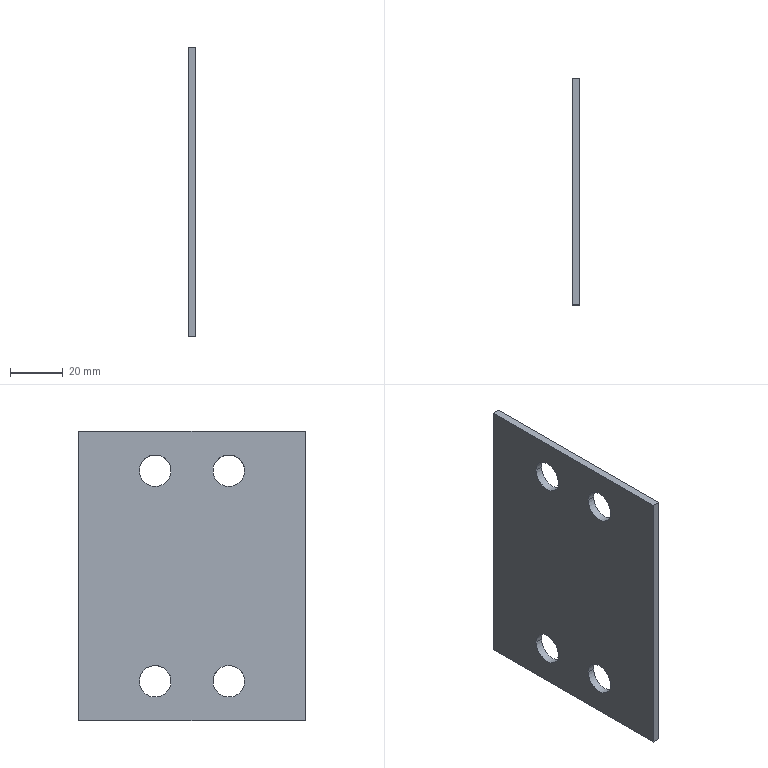Part | STEP file | Positioning_id1982_x_t | 1 solid | 14 faces | box 3 x 86 x 110 mm | volume 27023 mm3 | cylinder 8 | plane 6 | commonest cylinder face diameters 12 x8
STEP:
#1=CARTESIAN_POINT('',(0.,0.,0.));
#2=DIRECTION('',(0.,0.,1.));
#3=DIRECTION('',(1.,0.,0.));
#4=AXIS2_PLACEMENT_3D('',#1,#2,#3);
#5=CARTESIAN_POINT('',(-1013.002,8.,316.5));
#6=VERTEX_POINT('',#5);
#7=CARTESIAN_POINT('',(-1013.002,20.,316.5));
#8=VERTEX_POINT('',#7);
#9=CARTESIAN_POINT('',(-1013.002,14.,316.5));
#10=DIRECTION('',(1.,0.,0.));
#11=DIRECTION('',(0.,0.,-1.));
#12=AXIS2_PLACEMENT_3D('',#9,#10,#11);
#13=CIRCLE('',#12,6.);
#14=CARTESIAN_POINT('',(-995.002,14.,316.5));
#15=DIRECTION('',(1.,0.,0.));
#16=DIRECTION('',(0.,-1.,0.));
#17=AXIS2_PLACEMENT_3D('',#14,#15,#16);
#18=CYLINDRICAL_SURFACE('',#17,6.);
#19=CARTESIAN_POINT('',(-4.712,-18.));
#20=DIRECTION('',(1.,0.));
#21=VECTOR('',#20,1.);
#22=LINE('',#19,#21);
#23=(GEOMETRIC_REPRESENTATION_CONTEXT(2)PARAMETRIC_REPRESENTATION_CONTEXT()REPRESENTATION_CONTEXT('',''));
#24=DEFINITIONAL_REPRESENTATION('',(#22),#23);
#25=PCURVE('',#18,#24);
#26=CARTESIAN_POINT('',(-1013.002,-74.25,599.5));
#27=DIRECTION('',(1.,0.,0.));
#28=DIRECTION('',(0.,1.,0.));
#29=AXIS2_PLACEMENT_3D('',#26,#27,#28);
#30=PLANE('',#29);
#31=CARTESIAN_POINT('',(88.25,-283.));
#32=DIRECTION('',(0.,-1.));
#33=AXIS2_PLACEMENT_2D('',#31,#32);
#34=CIRCLE('',#33,6.);
#35=(GEOMETRIC_REPRESENTATION_CONTEXT(2)PARAMETRIC_REPRESENTATION_CONTEXT()REPRESENTATION_CONTEXT('',''));
#36=DEFINITIONAL_REPRESENTATION('',(#34),#35);
#37=PCURVE('',#30,#36);
#38=SURFACE_CURVE('',#13,(#25,#37),.PCURVE_S1.);
#39=EDGE_CURVE('',#6,#8,#38,.T.);
#40=ORIENTED_EDGE('',*,*,#39,.T.);
#41=CARTESIAN_POINT('',(-1010.002,20.,316.5));
#42=VERTEX_POINT('',#41);
#43=CARTESIAN_POINT('',(-1010.002,20.,316.5));
#44=DIRECTION('',(-1.,0.,0.));
#45=VECTOR('',#44,1.);
#46=LINE('',#43,#45);
#47=CARTESIAN_POINT('',(3.142,-15.));
#48=DIRECTION('',(0.,-1.));
#49=VECTOR('',#48,1.);
#50=LINE('',#47,#49);
#51=(GEOMETRIC_REPRESENTATION_CONTEXT(2)PARAMETRIC_REPRESENTATION_CONTEXT()REPRESENTATION_CONTEXT('',''));
#52=DEFINITIONAL_REPRESENTATION('',(#50),#51);
#53=PCURVE('',#18,#52);
#54=CARTESIAN_POINT('',(-995.002,14.,316.5));
#55=DIRECTION('',(1.,0.,0.));
#56=DIRECTION('',(0.,-1.,0.));
#57=AXIS2_PLACEMENT_3D('',#54,#55,#56);
#58=CYLINDRICAL_SURFACE('',#57,6.);
#59=CARTESIAN_POINT('',(3.142,-15.));
#60=DIRECTION('',(0.,-1.));
#61=VECTOR('',#60,1.);
#62=LINE('',#59,#61);
#63=(GEOMETRIC_REPRESENTATION_CONTEXT(2)PARAMETRIC_REPRESENTATION_CONTEXT()REPRESENTATION_CONTEXT('',''));
#64=DEFINITIONAL_REPRESENTATION('',(#62),#63);
#65=PCURVE('',#58,#64);
#66=SURFACE_CURVE('',#46,(#53,#65),.PCURVE_S1.);
#67=EDGE_CURVE('',#42,#8,#66,.T.);
#68=ORIENTED_EDGE('',*,*,#67,.F.);
#69=CARTESIAN_POINT('',(-1010.002,8.,316.5));
#70=VERTEX_POINT('',#69);
#71=CARTESIAN_POINT('',(-1010.002,14.,316.5));
#72=DIRECTION('',(-1.,0.,0.));
#73=DIRECTION('',(0.,0.,-1.));
#74=AXIS2_PLACEMENT_3D('',#71,#72,#73);
#75=CIRCLE('',#74,6.);
#76=CARTESIAN_POINT('',(7.854,-15.));
#77=DIRECTION('',(-1.,0.));
#78=VECTOR('',#77,1.);
#79=LINE('',#76,#78);
#80=(GEOMETRIC_REPRESENTATION_CONTEXT(2)PARAMETRIC_REPRESENTATION_CONTEXT()REPRESENTATION_CONTEXT('',''));
#81=DEFINITIONAL_REPRESENTATION('',(#79),#80);
#82=PCURVE('',#18,#81);
#83=CARTESIAN_POINT('',(-1010.002,-29.,411.5));
#84=DIRECTION('',(1.,0.,0.));
#85=DIRECTION('',(0.,1.,0.));
#86=AXIS2_PLACEMENT_3D('',#83,#84,#85);
#87=PLANE('',#86);
#88=CARTESIAN_POINT('',(43.,-101.));
#89=CARTESIAN_POINT('',(32.608,-101.));
#90=CARTESIAN_POINT('',(37.804,-92.));
#91=CARTESIAN_POINT('',(43.,-83.));
#92=CARTESIAN_POINT('',(48.196,-92.));
#93=CARTESIAN_POINT('',(53.392,-101.));
#94=CARTESIAN_POINT('',(43.,-101.));
#95=(BOUNDED_CURVE()B_SPLINE_CURVE(2,(#88,#89,#90,#91,#92,#93,#94),.UNSPECIFIED.,.T.,.F.)B_SPLINE_CURVE_WITH_KNOTS((1,2,2,2,2,1),(-2.094,0.,2.094,4.189,6.283,8.378),.UNSPECIFIED.)CURVE()GEOMETRIC_REPRESENTATION_ITEM()RATIONAL_B_SPLINE_CURVE((1.,0.5,1.,0.5,1.,0.5,1.))REPRESENTATION_ITEM(''));
#96=(GEOMETRIC_REPRESENTATION_CONTEXT(2)PARAMETRIC_REPRESENTATION_CONTEXT()REPRESENTATION_CONTEXT('',''));
#97=DEFINITIONAL_REPRESENTATION('',(#95),#96);
#98=PCURVE('',#87,#97);
#99=SURFACE_CURVE('',#75,(#82,#98),.PCURVE_S1.);
#100=EDGE_CURVE('',#42,#70,#99,.T.);
#101=ORIENTED_EDGE('',*,*,#100,.T.);
#102=CARTESIAN_POINT('',(-1010.002,8.,316.5));
#103=DIRECTION('',(1.,0.,0.));
#104=VECTOR('',#103,1.);
#105=LINE('',#102,#104);
#106=CARTESIAN_POINT('',(0.,-15.));
#107=DIRECTION('',(0.,1.));
#108=VECTOR('',#107,1.);
#109=LINE('',#106,#108);
#110=(GEOMETRIC_REPRESENTATION_CONTEXT(2)PARAMETRIC_REPRESENTATION_CONTEXT()REPRESENTATION_CONTEXT('',''));
#111=DEFINITIONAL_REPRESENTATION('',(#109),#110);
#112=PCURVE('',#18,#111);
#113=CARTESIAN_POINT('',(6.283,-15.));
#114=DIRECTION('',(0.,1.));
#115=VECTOR('',#114,1.);
#116=LINE('',#113,#115);
#117=(GEOMETRIC_REPRESENTATION_CONTEXT(2)PARAMETRIC_REPRESENTATION_CONTEXT()REPRESENTATION_CONTEXT('',''));
#118=DEFINITIONAL_REPRESENTATION('',(#116),#117);
#119=PCURVE('',#58,#118);
#120=SURFACE_CURVE('',#105,(#112,#119),.PCURVE_S1.);
#121=EDGE_CURVE('',#6,#70,#120,.T.);
#122=ORIENTED_EDGE('',*,*,#121,.F.);
#123=EDGE_LOOP('',(#40,#68,#101,#122));
#124=FACE_BOUND('',#123,.F.);
#125=ADVANCED_FACE('',(#124),#18,.F.);
#126=CARTESIAN_POINT('',(-1013.002,-8.,316.5));
#127=VERTEX_POINT('',#126);
#128=CARTESIAN_POINT('',(-1013.002,-20.,316.5));
#129=VERTEX_POINT('',#128);
#130=CARTESIAN_POINT('',(-1013.002,-14.,316.5));
#131=DIRECTION('',(1.,0.,0.));
#132=DIRECTION('',(0.,1.,0.));
#133=AXIS2_PLACEMENT_3D('',#130,#131,#132);
#134=CIRCLE('',#133,6.);
#135=CARTESIAN_POINT('',(60.25,-283.));
#136=DIRECTION('',(1.,0.));
#137=AXIS2_PLACEMENT_2D('',#135,#136);
#138=CIRCLE('',#137,6.);
#139=(GEOMETRIC_REPRESENTATION_CONTEXT(2)PARAMETRIC_REPRESENTATION_CONTEXT()REPRESENTATION_CONTEXT('',''));
#140=DEFINITIONAL_REPRESENTATION('',(#138),#139);
#141=PCURVE('',#30,#140);
#142=CARTESIAN_POINT('',(-995.002,-14.,316.5));
#143=DIRECTION('',(1.,0.,0.));
#144=DIRECTION('',(0.,-1.,0.));
#145=AXIS2_PLACEMENT_3D('',#142,#143,#144);
#146=CYLINDRICAL_SURFACE('',#145,6.);
#147=CARTESIAN_POINT('',(3.142,-18.));
#148=DIRECTION('',(1.,0.));
#149=VECTOR('',#148,1.);
#150=LINE('',#147,#149);
#151=(GEOMETRIC_REPRESENTATION_CONTEXT(2)PARAMETRIC_REPRESENTATION_CONTEXT()REPRESENTATION_CONTEXT('',''));
#152=DEFINITIONAL_REPRESENTATION('',(#150),#151);
#153=PCURVE('',#146,#152);
#154=SURFACE_CURVE('',#134,(#141,#153),.PCURVE_S1.);
#155=EDGE_CURVE('',#127,#129,#154,.T.);
#156=ORIENTED_EDGE('',*,*,#155,.T.);
#157=CARTESIAN_POINT('',(-1013.002,-14.,316.5));
#158=DIRECTION('',(1.,0.,0.));
#159=DIRECTION('',(0.,-1.,0.));
#160=AXIS2_PLACEMENT_3D('',#157,#158,#159);
#161=CIRCLE('',#160,6.);
#162=CARTESIAN_POINT('',(60.25,-283.));
#163=DIRECTION('',(-1.,0.));
#164=AXIS2_PLACEMENT_2D('',#162,#163);
#165=CIRCLE('',#164,6.);
#166=(GEOMETRIC_REPRESENTATION_CONTEXT(2)PARAMETRIC_REPRESENTATION_CONTEXT()REPRESENTATION_CONTEXT('',''));
#167=DEFINITIONAL_REPRESENTATION('',(#165),#166);
#168=PCURVE('',#30,#167);
#169=CARTESIAN_POINT('',(-995.002,-14.,316.5));
#170=DIRECTION('',(1.,0.,0.));
#171=DIRECTION('',(0.,-1.,0.));
#172=AXIS2_PLACEMENT_3D('',#169,#170,#171);
#173=CYLINDRICAL_SURFACE('',#172,6.);
#174=CARTESIAN_POINT('',(0.,-18.));
#175=DIRECTION('',(1.,0.));
#176=VECTOR('',#175,1.);
#177=LINE('',#174,#176);
#178=(GEOMETRIC_REPRESENTATION_CONTEXT(2)PARAMETRIC_REPRESENTATION_CONTEXT()REPRESENTATION_CONTEXT('',''));
#179=DEFINITIONAL_REPRESENTATION('',(#177),#178);
#180=PCURVE('',#173,#179);
#181=SURFACE_CURVE('',#161,(#168,#180),.PCURVE_S1.);
#182=EDGE_CURVE('',#129,#127,#181,.T.);
#183=ORIENTED_EDGE('',*,*,#182,.T.);
#184=EDGE_LOOP('',(#156,#183));
#185=FACE_BOUND('',#184,.T.);
#186=CARTESIAN_POINT('',(-1013.002,20.,316.5));
#187=CARTESIAN_POINT('',(-1013.002,20.,322.5));
#188=CARTESIAN_POINT('',(-1013.002,14.,325.5));
#189=CARTESIAN_POINT('',(-1013.002,8.,322.5));
#190=CARTESIAN_POINT('',(-1013.002,8.,316.5));
#191=(BOUNDED_CURVE()B_SPLINE_CURVE(4,(#186,#187,#188,#189,#190),.UNSPECIFIED.,.F.,.F.)B_SPLINE_CURVE_WITH_KNOTS((5,5),(0.,1.),.PIECEWISE_BEZIER_KNOTS.)CURVE()GEOMETRIC_REPRESENTATION_ITEM()RATIONAL_B_SPLINE_CURVE((1.,0.7071,0.6667,0.7071,1.))REPRESENTATION_ITEM(''));
#192=CARTESIAN_POINT('',(94.25,-283.));
#193=CARTESIAN_POINT('',(94.25,-277.));
#194=CARTESIAN_POINT('',(88.25,-274.));
#195=CARTESIAN_POINT('',(82.25,-277.));
#196=CARTESIAN_POINT('',(82.25,-283.));
#197=(BOUNDED_CURVE()B_SPLINE_CURVE(4,(#192,#193,#194,#195,#196),.UNSPECIFIED.,.F.,.F.)B_SPLINE_CURVE_WITH_KNOTS((5,5),(0.,1.),.PIECEWISE_BEZIER_KNOTS.)CURVE()GEOMETRIC_REPRESENTATION_ITEM()RATIONAL_B_SPLINE_CURVE((1.,0.7071,0.6667,0.7071,1.))REPRESENTATION_ITEM(''));
#198=(GEOMETRIC_REPRESENTATION_CONTEXT(2)PARAMETRIC_REPRESENTATION_CONTEXT()REPRESENTATION_CONTEXT('',''));
#199=DEFINITIONAL_REPRESENTATION('',(#197),#198);
#200=PCURVE('',#30,#199);
#201=CARTESIAN_POINT('',(3.142,-18.));
#202=CARTESIAN_POINT('',(3.184,-18.));
#203=CARTESIAN_POINT('',(3.271,-18.));
#204=CARTESIAN_POINT('',(3.405,-18.));
#205=CARTESIAN_POINT('',(3.542,-18.));
#206=CARTESIAN_POINT('',(3.681,-18.));
#207=CARTESIAN_POINT('',(3.823,-18.));
#208=CARTESIAN_POINT('',(3.968,-18.));
#209=CARTESIAN_POINT('',(4.114,-18.));
#210=CARTESIAN_POINT('',(4.262,-18.));
#211=CARTESIAN_POINT('',(4.412,-18.));
#212=CARTESIAN_POINT('',(4.562,-18.));
#213=CARTESIAN_POINT('',(4.712,-18.));
#214=CARTESIAN_POINT('',(4.863,-18.));
#215=CARTESIAN_POINT('',(5.013,-18.));
#216=CARTESIAN_POINT('',(5.163,-18.));
#217=CARTESIAN_POINT('',(5.311,-18.));
#218=CARTESIAN_POINT('',(5.457,-18.));
#219=CARTESIAN_POINT('',(5.602,-18.));
#220=CARTESIAN_POINT('',(5.744,-18.));
#221=CARTESIAN_POINT('',(5.883,-18.));
#222=CARTESIAN_POINT('',(6.02,-18.));
#223=CARTESIAN_POINT('',(6.153,-18.));
#224=CARTESIAN_POINT('',(6.24,-18.));
#225=CARTESIAN_POINT('',(6.283,-18.));
#226=B_SPLINE_CURVE_WITH_KNOTS('',3,(#201,#202,#203,#204,#205,#206,#207,#208,#209,#210,#211,#212,#213,#214,#215,#216,#217,#218,#219,#220,#221,#222,#223,#224,#225),.UNSPECIFIED.,.F.,.F.,(4,1,1,1,1,1,1,1,1,1,1,1,1,1,1,1,1,1,1,1,1,1,4),(0.,0.04545,0.09091,0.1364,0.1818,0.2273,0.2727,0.3182,0.3636,0.4091,0.4545,0.5,0.5455,0.5909,0.6364,0.6818,0.7273,0.7727,0.8182,0.8636,0.9091,0.9545,1.),.QUASI_UNIFORM_KNOTS.);
#227=(GEOMETRIC_REPRESENTATION_CONTEXT(2)PARAMETRIC_REPRESENTATION_CONTEXT()REPRESENTATION_CONTEXT('',''));
#228=DEFINITIONAL_REPRESENTATION('',(#226),#227);
#229=PCURVE('',#58,#228);
#230=SURFACE_CURVE('',#191,(#200,#229),.PCURVE_S1.);
#231=EDGE_CURVE('',#8,#6,#230,.T.);
#232=ORIENTED_EDGE('',*,*,#231,.T.);
#233=ORIENTED_EDGE('',*,*,#39,.T.);
#234=EDGE_LOOP('',(#232,#233));
#235=FACE_BOUND('',#234,.T.);
#236=CARTESIAN_POINT('',(-1013.002,-8.,396.5));
#237=VERTEX_POINT('',#236);
#238=CARTESIAN_POINT('',(-1013.002,-20.,396.5));
#239=VERTEX_POINT('',#238);
#240=CARTESIAN_POINT('',(-1013.002,-14.,396.5));
#241=DIRECTION('',(-1.,0.,0.));
#242=DIRECTION('',(0.,1.,0.));
#243=AXIS2_PLACEMENT_3D('',#240,#241,#242);
#244=CIRCLE('',#243,6.);
#245=CARTESIAN_POINT('',(66.25,-203.));
#246=CARTESIAN_POINT('',(66.25,-213.392));
#247=CARTESIAN_POINT('',(57.25,-208.196));
#248=CARTESIAN_POINT('',(48.25,-203.));
#249=CARTESIAN_POINT('',(57.25,-197.804));
#250=CARTESIAN_POINT('',(66.25,-192.608));
#251=CARTESIAN_POINT('',(66.25,-203.));
#252=(BOUNDED_CURVE()B_SPLINE_CURVE(2,(#245,#246,#247,#248,#249,#250,#251),.UNSPECIFIED.,.T.,.F.)B_SPLINE_CURVE_WITH_KNOTS((1,2,2,2,2,1),(-2.094,0.,2.094,4.189,6.283,8.378),.UNSPECIFIED.)CURVE()GEOMETRIC_REPRESENTATION_ITEM()RATIONAL_B_SPLINE_CURVE((1.,0.5,1.,0.5,1.,0.5,1.))REPRESENTATION_ITEM(''));
#253=(GEOMETRIC_REPRESENTATION_CONTEXT(2)PARAMETRIC_REPRESENTATION_CONTEXT()REPRESENTATION_CONTEXT('',''));
#254=DEFINITIONAL_REPRESENTATION('',(#252),#253);
#255=PCURVE('',#30,#254);
#256=CARTESIAN_POINT('',(-995.002,-14.,396.5));
#257=DIRECTION('',(1.,0.,0.));
#258=DIRECTION('',(0.,-1.,0.));
#259=AXIS2_PLACEMENT_3D('',#256,#257,#258);
#260=CYLINDRICAL_SURFACE('',#259,6.);
#261=CARTESIAN_POINT('',(3.142,-18.));
#262=DIRECTION('',(-1.,0.));
#263=VECTOR('',#262,1.);
#264=LINE('',#261,#263);
#265=(GEOMETRIC_REPRESENTATION_CONTEXT(2)PARAMETRIC_REPRESENTATION_CONTEXT()REPRESENTATION_CONTEXT('',''));
#266=DEFINITIONAL_REPRESENTATION('',(#264),#265);
#267=PCURVE('',#260,#266);
#268=SURFACE_CURVE('',#244,(#255,#267),.PCURVE_S1.);
#269=EDGE_CURVE('',#237,#239,#268,.T.);
#270=ORIENTED_EDGE('',*,*,#269,.F.);
#271=CARTESIAN_POINT('',(-1013.002,-14.,396.5));
#272=DIRECTION('',(-1.,0.,0.));
#273=DIRECTION('',(0.,-1.,0.));
#274=AXIS2_PLACEMENT_3D('',#271,#272,#273);
#275=CIRCLE('',#274,6.);
#276=CARTESIAN_POINT('',(54.25,-203.));
#277=CARTESIAN_POINT('',(54.25,-192.608));
#278=CARTESIAN_POINT('',(63.25,-197.804));
#279=CARTESIAN_POINT('',(72.25,-203.));
#280=CARTESIAN_POINT('',(63.25,-208.196));
#281=CARTESIAN_POINT('',(54.25,-213.392));
#282=CARTESIAN_POINT('',(54.25,-203.));
#283=(BOUNDED_CURVE()B_SPLINE_CURVE(2,(#276,#277,#278,#279,#280,#281,#282),.UNSPECIFIED.,.T.,.F.)B_SPLINE_CURVE_WITH_KNOTS((1,2,2,2,2,1),(-2.094,0.,2.094,4.189,6.283,8.378),.UNSPECIFIED.)CURVE()GEOMETRIC_REPRESENTATION_ITEM()RATIONAL_B_SPLINE_CURVE((1.,0.5,1.,0.5,1.,0.5,1.))REPRESENTATION_ITEM(''));
#284=(GEOMETRIC_REPRESENTATION_CONTEXT(2)PARAMETRIC_REPRESENTATION_CONTEXT()REPRESENTATION_CONTEXT('',''));
#285=DEFINITIONAL_REPRESENTATION('',(#283),#284);
#286=PCURVE('',#30,#285);
#287=CARTESIAN_POINT('',(-995.002,-14.,396.5));
#288=DIRECTION('',(1.,0.,0.));
#289=DIRECTION('',(0.,-1.,0.));
#290=AXIS2_PLACEMENT_3D('',#287,#288,#289);
#291=CYLINDRICAL_SURFACE('',#290,6.);
#292=CARTESIAN_POINT('',(6.283,-18.));
#293=DIRECTION('',(-1.,0.));
#294=VECTOR('',#293,1.);
#295=LINE('',#292,#294);
#296=(GEOMETRIC_REPRESENTATION_CONTEXT(2)PARAMETRIC_REPRESENTATION_CONTEXT()REPRESENTATION_CONTEXT('',''));
#297=DEFINITIONAL_REPRESENTATION('',(#295),#296);
#298=PCURVE('',#291,#297);
#299=SURFACE_CURVE('',#275,(#286,#298),.PCURVE_S1.);
#300=EDGE_CURVE('',#239,#237,#299,.T.);
#301=ORIENTED_EDGE('',*,*,#300,.F.);
#302=EDGE_LOOP('',(#270,#301));
#303=FACE_BOUND('',#302,.T.);
#304=CARTESIAN_POINT('',(-1013.002,20.,396.5));
#305=VERTEX_POINT('',#304);
#306=CARTESIAN_POINT('',(-1013.002,8.,396.5));
#307=VERTEX_POINT('',#306);
#308=CARTESIAN_POINT('',(-1013.002,14.,396.5));
#309=DIRECTION('',(-1.,0.,0.));
#310=DIRECTION('',(0.,1.,0.));
#311=AXIS2_PLACEMENT_3D('',#308,#309,#310);
#312=CIRCLE('',#311,6.);
#313=CARTESIAN_POINT('',(94.25,-203.));
#314=CARTESIAN_POINT('',(94.25,-213.392));
#315=CARTESIAN_POINT('',(85.25,-208.196));
#316=CARTESIAN_POINT('',(76.25,-203.));
#317=CARTESIAN_POINT('',(85.25,-197.804));
#318=CARTESIAN_POINT('',(94.25,-192.608));
#319=CARTESIAN_POINT('',(94.25,-203.));
#320=(BOUNDED_CURVE()B_SPLINE_CURVE(2,(#313,#314,#315,#316,#317,#318,#319),.UNSPECIFIED.,.T.,.F.)B_SPLINE_CURVE_WITH_KNOTS((1,2,2,2,2,1),(-2.094,0.,2.094,4.189,6.283,8.378),.UNSPECIFIED.)CURVE()GEOMETRIC_REPRESENTATION_ITEM()RATIONAL_B_SPLINE_CURVE((1.,0.5,1.,0.5,1.,0.5,1.))REPRESENTATION_ITEM(''));
#321=(GEOMETRIC_REPRESENTATION_CONTEXT(2)PARAMETRIC_REPRESENTATION_CONTEXT()REPRESENTATION_CONTEXT('',''));
#322=DEFINITIONAL_REPRESENTATION('',(#320),#321);
#323=PCURVE('',#30,#322);
#324=CARTESIAN_POINT('',(-995.002,14.,396.5));
#325=DIRECTION('',(1.,0.,0.));
#326=DIRECTION('',(0.,-1.,0.));
#327=AXIS2_PLACEMENT_3D('',#324,#325,#326);
#328=CYLINDRICAL_SURFACE('',#327,6.);
#329=CARTESIAN_POINT('',(3.142,-18.));
#330=DIRECTION('',(-1.,0.));
#331=VECTOR('',#330,1.);
#332=LINE('',#329,#331);
#333=(GEOMETRIC_REPRESENTATION_CONTEXT(2)PARAMETRIC_REPRESENTATION_CONTEXT()REPRESENTATION_CONTEXT('',''));
#334=DEFINITIONAL_REPRESENTATION('',(#332),#333);
#335=PCURVE('',#328,#334);
#336=SURFACE_CURVE('',#312,(#323,#335),.PCURVE_S1.);
#337=EDGE_CURVE('',#305,#307,#336,.T.);
#338=ORIENTED_EDGE('',*,*,#337,.F.);
#339=CARTESIAN_POINT('',(-1013.002,14.,396.5));
#340=DIRECTION('',(-1.,0.,0.));
#341=DIRECTION('',(0.,-1.,0.));
#342=AXIS2_PLACEMENT_3D('',#339,#340,#341);
#343=CIRCLE('',#342,6.);
#344=CARTESIAN_POINT('',(82.25,-203.));
#345=CARTESIAN_POINT('',(82.25,-192.608));
#346=CARTESIAN_POINT('',(91.25,-197.804));
#347=CARTESIAN_POINT('',(100.25,-203.));
#348=CARTESIAN_POINT('',(91.25,-208.196));
#349=CARTESIAN_POINT('',(82.25,-213.392));
#350=CARTESIAN_POINT('',(82.25,-203.));
#351=(BOUNDED_CURVE()B_SPLINE_CURVE(2,(#344,#345,#346,#347,#348,#349,#350),.UNSPECIFIED.,.T.,.F.)B_SPLINE_CURVE_WITH_KNOTS((1,2,2,2,2,1),(-2.094,0.,2.094,4.189,6.283,8.378),.UNSPECIFIED.)CURVE()GEOMETRIC_REPRESENTATION_ITEM()RATIONAL_B_SPLINE_CURVE((1.,0.5,1.,0.5,1.,0.5,1.))REPRESENTATION_ITEM(''));
#352=(GEOMETRIC_REPRESENTATION_CONTEXT(2)PARAMETRIC_REPRESENTATION_CONTEXT()REPRESENTATION_CONTEXT('',''));
#353=DEFINITIONAL_REPRESENTATION('',(#351),#352);
#354=PCURVE('',#30,#353);
#355=CARTESIAN_POINT('',(-995.002,14.,396.5));
#356=DIRECTION('',(1.,0.,0.));
#357=DIRECTION('',(0.,-1.,0.));
#358=AXIS2_PLACEMENT_3D('',#355,#356,#357);
#359=CYLINDRICAL_SURFACE('',#358,6.);
#360=CARTESIAN_POINT('',(6.283,-18.));
#361=DIRECTION('',(-1.,0.));
#362=VECTOR('',#361,1.);
#363=LINE('',#360,#362);
#364=(GEOMETRIC_REPRESENTATION_CONTEXT(2)PARAMETRIC_REPRESENTATION_CONTEXT()REPRESENTATION_CONTEXT('',''));
#365=DEFINITIONAL_REPRESENTATION('',(#363),#364);
#366=PCURVE('',#359,#365);
#367=SURFACE_CURVE('',#343,(#354,#366),.PCURVE_S1.);
#368=EDGE_CURVE('',#307,#305,#367,.T.);
#369=ORIENTED_EDGE('',*,*,#368,.F.);
#370=EDGE_LOOP('',(#338,#369));
#371=FACE_BOUND('',#370,.T.);
#372=CARTESIAN_POINT('',(-1013.002,43.,301.5));
#373=VERTEX_POINT('',#372);
#374=CARTESIAN_POINT('',(-1013.002,43.,411.5));
#375=VERTEX_POINT('',#374);
#376=CARTESIAN_POINT('',(-1013.002,43.,301.5));
#377=DIRECTION('',(0.,0.,1.));
#378=VECTOR('',#377,1.);
#379=LINE('',#376,#378);
#380=CARTESIAN_POINT('',(117.25,-298.));
#381=DIRECTION('',(0.,1.));
#382=VECTOR('',#381,1.);
#383=LINE('',#380,#382);
#384=(GEOMETRIC_REPRESENTATION_CONTEXT(2)PARAMETRIC_REPRESENTATION_CONTEXT()REPRESENTATION_CONTEXT('',''));
#385=DEFINITIONAL_REPRESENTATION('',(#383),#384);
#386=PCURVE('',#30,#385);
#387=CARTESIAN_POINT('',(-1013.002,43.,336.5));
#388=DIRECTION('',(0.,1.,0.));
#389=DIRECTION('',(-1.,0.,0.));
#390=AXIS2_PLACEMENT_3D('',#387,#388,#389);
#391=PLANE('',#390);
#392=CARTESIAN_POINT('',(0.,-35.));
#393=DIRECTION('',(0.,1.));
#394=VECTOR('',#393,1.);
#395=LINE('',#392,#394);
#396=(GEOMETRIC_REPRESENTATION_CONTEXT(2)PARAMETRIC_REPRESENTATION_CONTEXT()REPRESENTATION_CONTEXT('',''));
#397=DEFINITIONAL_REPRESENTATION('',(#395),#396);
#398=PCURVE('',#391,#397);
#399=SURFACE_CURVE('',#379,(#386,#398),.PCURVE_S1.);
#400=EDGE_CURVE('',#373,#375,#399,.T.);
#401=ORIENTED_EDGE('',*,*,#400,.F.);
#402=CARTESIAN_POINT('',(-1013.002,-43.,301.5));
#403=VERTEX_POINT('',#402);
#404=CARTESIAN_POINT('',(-1013.002,43.,301.5));
#405=DIRECTION('',(0.,-1.,0.));
#406=VECTOR('',#405,1.);
#407=LINE('',#404,#406);
#408=CARTESIAN_POINT('',(117.25,-298.));
#409=DIRECTION('',(-1.,0.));
#410=VECTOR('',#409,1.);
#411=LINE('',#408,#410);
#412=(GEOMETRIC_REPRESENTATION_CONTEXT(2)PARAMETRIC_REPRESENTATION_CONTEXT()REPRESENTATION_CONTEXT('',''));
#413=DEFINITIONAL_REPRESENTATION('',(#411),#412);
#414=PCURVE('',#30,#413);
#415=CARTESIAN_POINT('',(-1006.775,-0.00002599,301.5));
#416=DIRECTION('',(0.,0.,-1.));
#417=DIRECTION('',(0.,-1.,0.));
#418=AXIS2_PLACEMENT_3D('',#415,#416,#417);
#419=PLANE('',#418);
#420=CARTESIAN_POINT('',(-43.,6.227));
#421=DIRECTION('',(1.,0.));
#422=VECTOR('',#421,1.);
#423=LINE('',#420,#422);
#424=(GEOMETRIC_REPRESENTATION_CONTEXT(2)PARAMETRIC_REPRESENTATION_CONTEXT()REPRESENTATION_CONTEXT('',''));
#425=DEFINITIONAL_REPRESENTATION('',(#423),#424);
#426=PCURVE('',#419,#425);
#427=SURFACE_CURVE('',#407,(#414,#426),.PCURVE_S1.);
#428=EDGE_CURVE('',#373,#403,#427,.T.);
#429=ORIENTED_EDGE('',*,*,#428,.T.);
#430=CARTESIAN_POINT('',(-1013.002,-43.,411.5));
#431=VERTEX_POINT('',#430);
#432=CARTESIAN_POINT('',(-1013.002,-43.,411.5));
#433=DIRECTION('',(0.,0.,-1.));
#434=VECTOR('',#433,1.);
#435=LINE('',#432,#434);
#436=CARTESIAN_POINT('',(31.25,-188.));
#437=DIRECTION('',(0.,-1.));
#438=VECTOR('',#437,1.);
#439=LINE('',#436,#438);
#440=(GEOMETRIC_REPRESENTATION_CONTEXT(2)PARAMETRIC_REPRESENTATION_CONTEXT()REPRESENTATION_CONTEXT('',''));
#441=DEFINITIONAL_REPRESENTATION('',(#439),#440);
#442=PCURVE('',#30,#441);
#443=CARTESIAN_POINT('',(-956.775,-43.,336.5));
#444=DIRECTION('',(0.,1.,0.));
#445=DIRECTION('',(-1.,0.,0.));
#446=AXIS2_PLACEMENT_3D('',#443,#444,#445);
#447=PLANE('',#446);
#448=CARTESIAN_POINT('',(56.227,75.));
#449=DIRECTION('',(0.,-1.));
#450=VECTOR('',#449,1.);
#451=LINE('',#448,#450);
#452=(GEOMETRIC_REPRESENTATION_CONTEXT(2)PARAMETRIC_REPRESENTATION_CONTEXT()REPRESENTATION_CONTEXT('',''));
#453=DEFINITIONAL_REPRESENTATION('',(#451),#452);
#454=PCURVE('',#447,#453);
#455=SURFACE_CURVE('',#435,(#442,#454),.PCURVE_S1.);
#456=EDGE_CURVE('',#431,#403,#455,.T.);
#457=ORIENTED_EDGE('',*,*,#456,.F.);
#458=CARTESIAN_POINT('',(-1013.002,43.,411.5));
#459=DIRECTION('',(0.,-1.,0.));
#460=VECTOR('',#459,1.);
#461=LINE('',#458,#460);
#462=CARTESIAN_POINT('',(117.25,-188.));
#463=DIRECTION('',(-1.,0.));
#464=VECTOR('',#463,1.);
#465=LINE('',#462,#464);
#466=(GEOMETRIC_REPRESENTATION_CONTEXT(2)PARAMETRIC_REPRESENTATION_CONTEXT()REPRESENTATION_CONTEXT('',''));
#467=DEFINITIONAL_REPRESENTATION('',(#465),#466);
#468=PCURVE('',#30,#467);
#469=CARTESIAN_POINT('',(-1006.775,-0.00002599,411.5));
#470=DIRECTION('',(0.,0.,1.));
#471=DIRECTION('',(0.,-1.,0.));
#472=AXIS2_PLACEMENT_3D('',#469,#470,#471);
#473=PLANE('',#472);
#474=CARTESIAN_POINT('',(-43.,-6.227));
#475=DIRECTION('',(1.,0.));
#476=VECTOR('',#475,1.);
#477=LINE('',#474,#476);
#478=(GEOMETRIC_REPRESENTATION_CONTEXT(2)PARAMETRIC_REPRESENTATION_CONTEXT()REPRESENTATION_CONTEXT('',''));
#479=DEFINITIONAL_REPRESENTATION('',(#477),#478);
#480=PCURVE('',#473,#479);
#481=SURFACE_CURVE('',#461,(#468,#480),.PCURVE_S1.);
#482=EDGE_CURVE('',#375,#431,#481,.T.);
#483=ORIENTED_EDGE('',*,*,#482,.F.);
#484=EDGE_LOOP('',(#401,#429,#457,#483));
#485=FACE_BOUND('',#484,.T.);
#486=ADVANCED_FACE('',(#185,#235,#303,#371,#485),#30,.F.);
#487=CARTESIAN_POINT('',(-1010.002,-43.,411.5));
#488=VERTEX_POINT('',#487);
#489=CARTESIAN_POINT('',(-1010.002,-43.,301.5));
#490=VERTEX_POINT('',#489);
#491=CARTESIAN_POINT('',(-1010.002,-43.,411.5));
#492=DIRECTION('',(0.,0.,-1.));
#493=VECTOR('',#492,1.);
#494=LINE('',#491,#493);
#495=CARTESIAN_POINT('',(53.227,75.));
#496=DIRECTION('',(0.,-1.));
#497=VECTOR('',#496,1.);
#498=LINE('',#495,#497);
#499=(GEOMETRIC_REPRESENTATION_CONTEXT(2)PARAMETRIC_REPRESENTATION_CONTEXT()REPRESENTATION_CONTEXT('',''));
#500=DEFINITIONAL_REPRESENTATION('',(#498),#499);
#501=PCURVE('',#447,#500);
#502=CARTESIAN_POINT('',(-14.,0.));
#503=DIRECTION('',(0.,-1.));
#504=VECTOR('',#503,1.);
#505=LINE('',#502,#504);
#506=(GEOMETRIC_REPRESENTATION_CONTEXT(2)PARAMETRIC_REPRESENTATION_CONTEXT()REPRESENTATION_CONTEXT('',''));
#507=DEFINITIONAL_REPRESENTATION('',(#505),#506);
#508=PCURVE('',#87,#507);
#509=SURFACE_CURVE('',#494,(#501,#508),.PCURVE_S1.);
#510=EDGE_CURVE('',#488,#490,#509,.T.);
#511=ORIENTED_EDGE('',*,*,#510,.F.);
#512=CARTESIAN_POINT('',(-1013.002,-43.,411.5));
#513=DIRECTION('',(1.,0.,0.));
#514=VECTOR('',#513,1.);
#515=LINE('',#512,#514);
#516=CARTESIAN_POINT('',(56.227,75.));
#517=DIRECTION('',(-1.,0.));
#518=VECTOR('',#517,1.);
#519=LINE('',#516,#518);
#520=(GEOMETRIC_REPRESENTATION_CONTEXT(2)PARAMETRIC_REPRESENTATION_CONTEXT()REPRESENTATION_CONTEXT('',''));
#521=DEFINITIONAL_REPRESENTATION('',(#519),#520);
#522=PCURVE('',#447,#521);
#523=CARTESIAN_POINT('',(43.,-6.227));
#524=DIRECTION('',(0.,1.));
#525=VECTOR('',#524,1.);
#526=LINE('',#523,#525);
#527=(GEOMETRIC_REPRESENTATION_CONTEXT(2)PARAMETRIC_REPRESENTATION_CONTEXT()REPRESENTATION_CONTEXT('',''));
#528=DEFINITIONAL_REPRESENTATION('',(#526),#527);
#529=PCURVE('',#473,#528);
#530=SURFACE_CURVE('',#515,(#522,#529),.PCURVE_S1.);
#531=EDGE_CURVE('',#431,#488,#530,.T.);
#532=ORIENTED_EDGE('',*,*,#531,.F.);
#533=ORIENTED_EDGE('',*,*,#456,.T.);
#534=CARTESIAN_POINT('',(-1013.002,-43.,301.5));
#535=DIRECTION('',(1.,0.,0.));
#536=VECTOR('',#535,1.);
#537=LINE('',#534,#536);
#538=CARTESIAN_POINT('',(56.227,-35.));
#539=DIRECTION('',(-1.,0.));
#540=VECTOR('',#539,1.);
#541=LINE('',#538,#540);
#542=(GEOMETRIC_REPRESENTATION_CONTEXT(2)PARAMETRIC_REPRESENTATION_CONTEXT()REPRESENTATION_CONTEXT('',''));
#543=DEFINITIONAL_REPRESENTATION('',(#541),#542);
#544=PCURVE('',#447,#543);
#545=CARTESIAN_POINT('',(43.,6.227));
#546=DIRECTION('',(0.,-1.));
#547=VECTOR('',#546,1.);
#548=LINE('',#545,#547);
#549=(GEOMETRIC_REPRESENTATION_CONTEXT(2)PARAMETRIC_REPRESENTATION_CONTEXT()REPRESENTATION_CONTEXT('',''));
#550=DEFINITIONAL_REPRESENTATION('',(#548),#549);
#551=PCURVE('',#419,#550);
#552=SURFACE_CURVE('',#537,(#544,#551),.PCURVE_S1.);
#553=EDGE_CURVE('',#403,#490,#552,.T.);
#554=ORIENTED_EDGE('',*,*,#553,.T.);
#555=EDGE_LOOP('',(#511,#532,#533,#554));
#556=FACE_BOUND('',#555,.T.);
#557=ADVANCED_FACE('',(#556),#447,.F.);
#558=CARTESIAN_POINT('',(-1010.002,43.,411.5));
#559=VERTEX_POINT('',#558);
#560=CARTESIAN_POINT('',(-1013.002,43.,411.5));
#561=DIRECTION('',(1.,0.,0.));
#562=VECTOR('',#561,1.);
#563=LINE('',#560,#562);
#564=CARTESIAN_POINT('',(0.,75.));
#565=DIRECTION('',(-1.,0.));
#566=VECTOR('',#565,1.);
#567=LINE('',#564,#566);
#568=(GEOMETRIC_REPRESENTATION_CONTEXT(2)PARAMETRIC_REPRESENTATION_CONTEXT()REPRESENTATION_CONTEXT('',''));
#569=DEFINITIONAL_REPRESENTATION('',(#567),#568);
#570=PCURVE('',#391,#569);
#571=CARTESIAN_POINT('',(-43.,-6.227));
#572=DIRECTION('',(0.,1.));
#573=VECTOR('',#572,1.);
#574=LINE('',#571,#573);
#575=(GEOMETRIC_REPRESENTATION_CONTEXT(2)PARAMETRIC_REPRESENTATION_CONTEXT()REPRESENTATION_CONTEXT('',''));
#576=DEFINITIONAL_REPRESENTATION('',(#574),#575);
#577=PCURVE('',#473,#576);
#578=SURFACE_CURVE('',#563,(#570,#577),.PCURVE_S1.);
#579=EDGE_CURVE('',#375,#559,#578,.T.);
#580=ORIENTED_EDGE('',*,*,#579,.T.);
#581=CARTESIAN_POINT('',(-1010.002,43.,301.5));
#582=VERTEX_POINT('',#581);
#583=CARTESIAN_POINT('',(-1010.002,43.,411.5));
#584=DIRECTION('',(0.,0.,-1.));
#585=VECTOR('',#584,1.);
#586=LINE('',#583,#585);
#587=CARTESIAN_POINT('',(-3.,75.));
#588=DIRECTION('',(0.,-1.));
#589=VECTOR('',#588,1.);
#590=LINE('',#587,#589);
#591=(GEOMETRIC_REPRESENTATION_CONTEXT(2)PARAMETRIC_REPRESENTATION_CONTEXT()REPRESENTATION_CONTEXT('',''));
#592=DEFINITIONAL_REPRESENTATION('',(#590),#591);
#593=PCURVE('',#391,#592);
#594=CARTESIAN_POINT('',(72.,0.));
#595=DIRECTION('',(0.,-1.));
#596=VECTOR('',#595,1.);
#597=LINE('',#594,#596);
#598=(GEOMETRIC_REPRESENTATION_CONTEXT(2)PARAMETRIC_REPRESENTATION_CONTEXT()REPRESENTATION_CONTEXT('',''));
#599=DEFINITIONAL_REPRESENTATION('',(#597),#598);
#600=PCURVE('',#87,#599);
#601=SURFACE_CURVE('',#586,(#593,#600),.PCURVE_S1.);
#602=EDGE_CURVE('',#559,#582,#601,.T.);
#603=ORIENTED_EDGE('',*,*,#602,.T.);
#604=CARTESIAN_POINT('',(-1013.002,43.,301.5));
#605=DIRECTION('',(1.,0.,0.));
#606=VECTOR('',#605,1.);
#607=LINE('',#604,#606);
#608=CARTESIAN_POINT('',(0.,-35.));
#609=DIRECTION('',(-1.,0.));
#610=VECTOR('',#609,1.);
#611=LINE('',#608,#610);
#612=(GEOMETRIC_REPRESENTATION_CONTEXT(2)PARAMETRIC_REPRESENTATION_CONTEXT()REPRESENTATION_CONTEXT('',''));
#613=DEFINITIONAL_REPRESENTATION('',(#611),#612);
#614=PCURVE('',#391,#613);
#615=CARTESIAN_POINT('',(-43.,6.227));
#616=DIRECTION('',(0.,-1.));
#617=VECTOR('',#616,1.);
#618=LINE('',#615,#617);
#619=(GEOMETRIC_REPRESENTATION_CONTEXT(2)PARAMETRIC_REPRESENTATION_CONTEXT()REPRESENTATION_CONTEXT('',''));
#620=DEFINITIONAL_REPRESENTATION('',(#618),#619);
#621=PCURVE('',#419,#620);
#622=SURFACE_CURVE('',#607,(#614,#621),.PCURVE_S1.);
#623=EDGE_CURVE('',#373,#582,#622,.T.);
#624=ORIENTED_EDGE('',*,*,#623,.F.);
#625=ORIENTED_EDGE('',*,*,#400,.T.);
#626=EDGE_LOOP('',(#580,#603,#624,#625));
#627=FACE_BOUND('',#626,.T.);
#628=ADVANCED_FACE('',(#627),#391,.T.);
#629=ORIENTED_EDGE('',*,*,#531,.T.);
#630=CARTESIAN_POINT('',(-1010.002,-43.,411.5));
#631=DIRECTION('',(0.,1.,0.));
#632=VECTOR('',#631,1.);
#633=LINE('',#630,#632);
#634=CARTESIAN_POINT('',(43.,-3.227));
#635=DIRECTION('',(-1.,0.));
#636=VECTOR('',#635,1.);
#637=LINE('',#634,#636);
#638=(GEOMETRIC_REPRESENTATION_CONTEXT(2)PARAMETRIC_REPRESENTATION_CONTEXT()REPRESENTATION_CONTEXT('',''));
#639=DEFINITIONAL_REPRESENTATION('',(#637),#638);
#640=PCURVE('',#473,#639);
#641=CARTESIAN_POINT('',(-14.,0.));
#642=DIRECTION('',(1.,0.));
#643=VECTOR('',#642,1.);
#644=LINE('',#641,#643);
#645=(GEOMETRIC_REPRESENTATION_CONTEXT(2)PARAMETRIC_REPRESENTATION_CONTEXT()REPRESENTATION_CONTEXT('',''));
#646=DEFINITIONAL_REPRESENTATION('',(#644),#645);
#647=PCURVE('',#87,#646);
#648=SURFACE_CURVE('',#633,(#640,#647),.PCURVE_S1.);
#649=EDGE_CURVE('',#488,#559,#648,.T.);
#650=ORIENTED_EDGE('',*,*,#649,.T.);
#651=ORIENTED_EDGE('',*,*,#579,.F.);
#652=ORIENTED_EDGE('',*,*,#482,.T.);
#653=EDGE_LOOP('',(#629,#650,#651,#652));
#654=FACE_BOUND('',#653,.T.);
#655=ADVANCED_FACE('',(#654),#473,.T.);
#656=ORIENTED_EDGE('',*,*,#623,.T.);
#657=CARTESIAN_POINT('',(-1010.002,43.,301.5));
#658=DIRECTION('',(0.,-1.,0.));
#659=VECTOR('',#658,1.);
#660=LINE('',#657,#659);
#661=CARTESIAN_POINT('',(-43.,3.227));
#662=DIRECTION('',(1.,0.));
#663=VECTOR('',#662,1.);
#664=LINE('',#661,#663);
#665=(GEOMETRIC_REPRESENTATION_CONTEXT(2)PARAMETRIC_REPRESENTATION_CONTEXT()REPRESENTATION_CONTEXT('',''));
#666=DEFINITIONAL_REPRESENTATION('',(#664),#665);
#667=PCURVE('',#419,#666);
#668=CARTESIAN_POINT('',(72.,-110.));
#669=DIRECTION('',(-1.,0.));
#670=VECTOR('',#669,1.);
#671=LINE('',#668,#670);
#672=(GEOMETRIC_REPRESENTATION_CONTEXT(2)PARAMETRIC_REPRESENTATION_CONTEXT()REPRESENTATION_CONTEXT('',''));
#673=DEFINITIONAL_REPRESENTATION('',(#671),#672);
#674=PCURVE('',#87,#673);
#675=SURFACE_CURVE('',#660,(#667,#674),.PCURVE_S1.);
#676=EDGE_CURVE('',#582,#490,#675,.T.);
#677=ORIENTED_EDGE('',*,*,#676,.T.);
#678=ORIENTED_EDGE('',*,*,#553,.F.);
#679=ORIENTED_EDGE('',*,*,#428,.F.);
#680=EDGE_LOOP('',(#656,#677,#678,#679));
#681=FACE_BOUND('',#680,.T.);
#682=ADVANCED_FACE('',(#681),#419,.T.);
#683=ORIENTED_EDGE('',*,*,#337,.F.);
#684=CARTESIAN_POINT('',(-1010.002,20.,396.5));
#685=VERTEX_POINT('',#684);
#686=CARTESIAN_POINT('',(-1010.002,20.,396.5));
#687=DIRECTION('',(1.,0.,0.));
#688=VECTOR('',#687,1.);
#689=LINE('',#686,#688);
#690=CARTESIAN_POINT('',(3.142,-15.));
#691=DIRECTION('',(0.,1.));
#692=VECTOR('',#691,1.);
#693=LINE('',#690,#692);
#694=(GEOMETRIC_REPRESENTATION_CONTEXT(2)PARAMETRIC_REPRESENTATION_CONTEXT()REPRESENTATION_CONTEXT('',''));
#695=DEFINITIONAL_REPRESENTATION('',(#693),#694);
#696=PCURVE('',#328,#695);
#697=CARTESIAN_POINT('',(3.142,-15.));
#698=DIRECTION('',(0.,1.));
#699=VECTOR('',#698,1.);
#700=LINE('',#697,#699);
#701=(GEOMETRIC_REPRESENTATION_CONTEXT(2)PARAMETRIC_REPRESENTATION_CONTEXT()REPRESENTATION_CONTEXT('',''));
#702=DEFINITIONAL_REPRESENTATION('',(#700),#701);
#703=PCURVE('',#359,#702);
#704=SURFACE_CURVE('',#689,(#696,#703),.PCURVE_S1.);
#705=EDGE_CURVE('',#305,#685,#704,.T.);
#706=ORIENTED_EDGE('',*,*,#705,.T.);
#707=CARTESIAN_POINT('',(-1010.002,8.,396.5));
#708=VERTEX_POINT('',#707);
#709=CARTESIAN_POINT('',(-1010.002,14.,396.5));
#710=DIRECTION('',(-1.,0.,0.));
#711=DIRECTION('',(0.,0.,-1.));
#712=AXIS2_PLACEMENT_3D('',#709,#710,#711);
#713=CIRCLE('',#712,6.);
#714=CARTESIAN_POINT('',(7.854,-15.));
#715=DIRECTION('',(-1.,0.));
#716=VECTOR('',#715,1.);
#717=LINE('',#714,#716);
#718=(GEOMETRIC_REPRESENTATION_CONTEXT(2)PARAMETRIC_REPRESENTATION_CONTEXT()REPRESENTATION_CONTEXT('',''));
#719=DEFINITIONAL_REPRESENTATION('',(#717),#718);
#720=PCURVE('',#328,#719);
#721=CARTESIAN_POINT('',(43.,-21.));
#722=CARTESIAN_POINT('',(32.608,-21.));
#723=CARTESIAN_POINT('',(37.804,-12.));
#724=CARTESIAN_POINT('',(43.,-3.));
#725=CARTESIAN_POINT('',(48.196,-12.));
#726=CARTESIAN_POINT('',(53.392,-21.));
#727=CARTESIAN_POINT('',(43.,-21.));
#728=(BOUNDED_CURVE()B_SPLINE_CURVE(2,(#721,#722,#723,#724,#725,#726,#727),.UNSPECIFIED.,.T.,.F.)B_SPLINE_CURVE_WITH_KNOTS((1,2,2,2,2,1),(-2.094,0.,2.094,4.189,6.283,8.378),.UNSPECIFIED.)CURVE()GEOMETRIC_REPRESENTATION_ITEM()RATIONAL_B_SPLINE_CURVE((1.,0.5,1.,0.5,1.,0.5,1.))REPRESENTATION_ITEM(''));
#729=(GEOMETRIC_REPRESENTATION_CONTEXT(2)PARAMETRIC_REPRESENTATION_CONTEXT()REPRESENTATION_CONTEXT('',''));
#730=DEFINITIONAL_REPRESENTATION('',(#728),#729);
#731=PCURVE('',#87,#730);
#732=SURFACE_CURVE('',#713,(#720,#731),.PCURVE_S1.);
#733=EDGE_CURVE('',#685,#708,#732,.T.);
#734=ORIENTED_EDGE('',*,*,#733,.T.);
#735=CARTESIAN_POINT('',(-1010.002,8.,396.5));
#736=DIRECTION('',(-1.,0.,0.));
#737=VECTOR('',#736,1.);
#738=LINE('',#735,#737);
#739=CARTESIAN_POINT('',(0.,-15.));
#740=DIRECTION('',(0.,-1.));
#741=VECTOR('',#740,1.);
#742=LINE('',#739,#741);
#743=(GEOMETRIC_REPRESENTATION_CONTEXT(2)PARAMETRIC_REPRESENTATION_CONTEXT()REPRESENTATION_CONTEXT('',''));
#744=DEFINITIONAL_REPRESENTATION('',(#742),#743);
#745=PCURVE('',#328,#744);
#746=CARTESIAN_POINT('',(6.283,-15.));
#747=DIRECTION('',(0.,-1.));
#748=VECTOR('',#747,1.);
#749=LINE('',#746,#748);
#750=(GEOMETRIC_REPRESENTATION_CONTEXT(2)PARAMETRIC_REPRESENTATION_CONTEXT()REPRESENTATION_CONTEXT('',''));
#751=DEFINITIONAL_REPRESENTATION('',(#749),#750);
#752=PCURVE('',#359,#751);
#753=SURFACE_CURVE('',#738,(#745,#752),.PCURVE_S1.);
#754=EDGE_CURVE('',#708,#307,#753,.T.);
#755=ORIENTED_EDGE('',*,*,#754,.T.);
#756=EDGE_LOOP('',(#683,#706,#734,#755));
#757=FACE_BOUND('',#756,.F.);
#758=ADVANCED_FACE('',(#757),#328,.F.);
#759=ORIENTED_EDGE('',*,*,#269,.F.);
#760=CARTESIAN_POINT('',(-1010.002,-8.,396.5));
#761=VERTEX_POINT('',#760);
#762=CARTESIAN_POINT('',(-1010.002,-8.,396.5));
#763=DIRECTION('',(-1.,0.,0.));
#764=VECTOR('',#763,1.);
#765=LINE('',#762,#764);
#766=CARTESIAN_POINT('',(3.142,-15.));
#767=DIRECTION('',(0.,-1.));
#768=VECTOR('',#767,1.);
#769=LINE('',#766,#768);
#770=(GEOMETRIC_REPRESENTATION_CONTEXT(2)PARAMETRIC_REPRESENTATION_CONTEXT()REPRESENTATION_CONTEXT('',''));
#771=DEFINITIONAL_REPRESENTATION('',(#769),#770);
#772=PCURVE('',#260,#771);
#773=CARTESIAN_POINT('',(3.142,-15.));
#774=DIRECTION('',(0.,-1.));
#775=VECTOR('',#774,1.);
#776=LINE('',#773,#775);
#777=(GEOMETRIC_REPRESENTATION_CONTEXT(2)PARAMETRIC_REPRESENTATION_CONTEXT()REPRESENTATION_CONTEXT('',''));
#778=DEFINITIONAL_REPRESENTATION('',(#776),#777);
#779=PCURVE('',#291,#778);
#780=SURFACE_CURVE('',#765,(#772,#779),.PCURVE_S1.);
#781=EDGE_CURVE('',#761,#237,#780,.T.);
#782=ORIENTED_EDGE('',*,*,#781,.F.);
#783=CARTESIAN_POINT('',(-1010.002,-20.,396.5));
#784=VERTEX_POINT('',#783);
#785=CARTESIAN_POINT('',(-1010.002,-14.,396.5));
#786=DIRECTION('',(-1.,0.,0.));
#787=DIRECTION('',(0.,0.,-1.));
#788=AXIS2_PLACEMENT_3D('',#785,#786,#787);
#789=CIRCLE('',#788,6.);
#790=CARTESIAN_POINT('',(7.854,-15.));
#791=DIRECTION('',(-1.,0.));
#792=VECTOR('',#791,1.);
#793=LINE('',#790,#792);
#794=(GEOMETRIC_REPRESENTATION_CONTEXT(2)PARAMETRIC_REPRESENTATION_CONTEXT()REPRESENTATION_CONTEXT('',''));
#795=DEFINITIONAL_REPRESENTATION('',(#793),#794);
#796=PCURVE('',#260,#795);
#797=CARTESIAN_POINT('',(15.,-21.));
#798=CARTESIAN_POINT('',(4.608,-21.));
#799=CARTESIAN_POINT('',(9.804,-12.));
#800=CARTESIAN_POINT('',(15.,-3.));
#801=CARTESIAN_POINT('',(20.196,-12.));
#802=CARTESIAN_POINT('',(25.392,-21.));
#803=CARTESIAN_POINT('',(15.,-21.));
#804=(BOUNDED_CURVE()B_SPLINE_CURVE(2,(#797,#798,#799,#800,#801,#802,#803),.UNSPECIFIED.,.T.,.F.)B_SPLINE_CURVE_WITH_KNOTS((1,2,2,2,2,1),(-2.094,0.,2.094,4.189,6.283,8.378),.UNSPECIFIED.)CURVE()GEOMETRIC_REPRESENTATION_ITEM()RATIONAL_B_SPLINE_CURVE((1.,0.5,1.,0.5,1.,0.5,1.))REPRESENTATION_ITEM(''));
#805=(GEOMETRIC_REPRESENTATION_CONTEXT(2)PARAMETRIC_REPRESENTATION_CONTEXT()REPRESENTATION_CONTEXT('',''));
#806=DEFINITIONAL_REPRESENTATION('',(#804),#805);
#807=PCURVE('',#87,#806);
#808=SURFACE_CURVE('',#789,(#796,#807),.PCURVE_S1.);
#809=EDGE_CURVE('',#761,#784,#808,.T.);
#810=ORIENTED_EDGE('',*,*,#809,.T.);
#811=CARTESIAN_POINT('',(-1010.002,-20.,396.5));
#812=DIRECTION('',(1.,0.,0.));
#813=VECTOR('',#812,1.);
#814=LINE('',#811,#813);
#815=CARTESIAN_POINT('',(0.,-15.));
#816=DIRECTION('',(0.,1.));
#817=VECTOR('',#816,1.);
#818=LINE('',#815,#817);
#819=(GEOMETRIC_REPRESENTATION_CONTEXT(2)PARAMETRIC_REPRESENTATION_CONTEXT()REPRESENTATION_CONTEXT('',''));
#820=DEFINITIONAL_REPRESENTATION('',(#818),#819);
#821=PCURVE('',#260,#820);
#822=CARTESIAN_POINT('',(6.283,-15.));
#823=DIRECTION('',(0.,1.));
#824=VECTOR('',#823,1.);
#825=LINE('',#822,#824);
#826=(GEOMETRIC_REPRESENTATION_CONTEXT(2)PARAMETRIC_REPRESENTATION_CONTEXT()REPRESENTATION_CONTEXT('',''));
#827=DEFINITIONAL_REPRESENTATION('',(#825),#826);
#828=PCURVE('',#291,#827);
#829=SURFACE_CURVE('',#814,(#821,#828),.PCURVE_S1.);
#830=EDGE_CURVE('',#239,#784,#829,.T.);
#831=ORIENTED_EDGE('',*,*,#830,.F.);
#832=EDGE_LOOP('',(#759,#782,#810,#831));
#833=FACE_BOUND('',#832,.F.);
#834=ADVANCED_FACE('',(#833),#260,.F.);
#835=ORIENTED_EDGE('',*,*,#182,.T.);
#836=CARTESIAN_POINT('',(-1010.002,-8.,316.5));
#837=VERTEX_POINT('',#836);
#838=CARTESIAN_POINT('',(-1010.002,-8.,316.5));
#839=DIRECTION('',(-1.,0.,0.));
#840=VECTOR('',#839,1.);
#841=LINE('',#838,#840);
#842=CARTESIAN_POINT('',(3.142,-15.));
#843=DIRECTION('',(0.,-1.));
#844=VECTOR('',#843,1.);
#845=LINE('',#842,#844);
#846=(GEOMETRIC_REPRESENTATION_CONTEXT(2)PARAMETRIC_REPRESENTATION_CONTEXT()REPRESENTATION_CONTEXT('',''));
#847=DEFINITIONAL_REPRESENTATION('',(#845),#846);
#848=PCURVE('',#173,#847);
#849=CARTESIAN_POINT('',(3.142,-15.));
#850=DIRECTION('',(0.,-1.));
#851=VECTOR('',#850,1.);
#852=LINE('',#849,#851);
#853=(GEOMETRIC_REPRESENTATION_CONTEXT(2)PARAMETRIC_REPRESENTATION_CONTEXT()REPRESENTATION_CONTEXT('',''));
#854=DEFINITIONAL_REPRESENTATION('',(#852),#853);
#855=PCURVE('',#146,#854);
#856=SURFACE_CURVE('',#841,(#848,#855),.PCURVE_S1.);
#857=EDGE_CURVE('',#837,#127,#856,.T.);
#858=ORIENTED_EDGE('',*,*,#857,.F.);
#859=CARTESIAN_POINT('',(-1010.002,-20.,316.5));
#860=VERTEX_POINT('',#859);
#861=CARTESIAN_POINT('',(-1010.002,-14.,316.5));
#862=DIRECTION('',(-1.,0.,0.));
#863=DIRECTION('',(0.,0.,-1.));
#864=AXIS2_PLACEMENT_3D('',#861,#862,#863);
#865=CIRCLE('',#864,6.);
#866=CARTESIAN_POINT('',(7.854,-15.));
#867=DIRECTION('',(-1.,0.));
#868=VECTOR('',#867,1.);
#869=LINE('',#866,#868);
#870=(GEOMETRIC_REPRESENTATION_CONTEXT(2)PARAMETRIC_REPRESENTATION_CONTEXT()REPRESENTATION_CONTEXT('',''));
#871=DEFINITIONAL_REPRESENTATION('',(#869),#870);
#872=PCURVE('',#173,#871);
#873=CARTESIAN_POINT('',(15.,-101.));
#874=CARTESIAN_POINT('',(4.608,-101.));
#875=CARTESIAN_POINT('',(9.804,-92.));
#876=CARTESIAN_POINT('',(15.,-83.));
#877=CARTESIAN_POINT('',(20.196,-92.));
#878=CARTESIAN_POINT('',(25.392,-101.));
#879=CARTESIAN_POINT('',(15.,-101.));
#880=(BOUNDED_CURVE()B_SPLINE_CURVE(2,(#873,#874,#875,#876,#877,#878,#879),.UNSPECIFIED.,.T.,.F.)B_SPLINE_CURVE_WITH_KNOTS((1,2,2,2,2,1),(-2.094,0.,2.094,4.189,6.283,8.378),.UNSPECIFIED.)CURVE()GEOMETRIC_REPRESENTATION_ITEM()RATIONAL_B_SPLINE_CURVE((1.,0.5,1.,0.5,1.,0.5,1.))REPRESENTATION_ITEM(''));
#881=(GEOMETRIC_REPRESENTATION_CONTEXT(2)PARAMETRIC_REPRESENTATION_CONTEXT()REPRESENTATION_CONTEXT('',''));
#882=DEFINITIONAL_REPRESENTATION('',(#880),#881);
#883=PCURVE('',#87,#882);
#884=SURFACE_CURVE('',#865,(#872,#883),.PCURVE_S1.);
#885=EDGE_CURVE('',#837,#860,#884,.T.);
#886=ORIENTED_EDGE('',*,*,#885,.T.);
#887=CARTESIAN_POINT('',(-1010.002,-20.,316.5));
#888=DIRECTION('',(1.,0.,0.));
#889=VECTOR('',#888,1.);
#890=LINE('',#887,#889);
#891=CARTESIAN_POINT('',(0.,-15.));
#892=DIRECTION('',(0.,1.));
#893=VECTOR('',#892,1.);
#894=LINE('',#891,#893);
#895=(GEOMETRIC_REPRESENTATION_CONTEXT(2)PARAMETRIC_REPRESENTATION_CONTEXT()REPRESENTATION_CONTEXT('',''));
#896=DEFINITIONAL_REPRESENTATION('',(#894),#895);
#897=PCURVE('',#173,#896);
#898=CARTESIAN_POINT('',(6.283,-15.));
#899=DIRECTION('',(0.,1.));
#900=VECTOR('',#899,1.);
#901=LINE('',#898,#900);
#902=(GEOMETRIC_REPRESENTATION_CONTEXT(2)PARAMETRIC_REPRESENTATION_CONTEXT()REPRESENTATION_CONTEXT('',''));
#903=DEFINITIONAL_REPRESENTATION('',(#901),#902);
#904=PCURVE('',#146,#903);
#905=SURFACE_CURVE('',#890,(#897,#904),.PCURVE_S1.);
#906=EDGE_CURVE('',#129,#860,#905,.T.);
#907=ORIENTED_EDGE('',*,*,#906,.F.);
#908=EDGE_LOOP('',(#835,#858,#886,#907));
#909=FACE_BOUND('',#908,.F.);
#910=ADVANCED_FACE('',(#909),#173,.F.);
#911=ORIENTED_EDGE('',*,*,#809,.T.);
#912=CARTESIAN_POINT('',(-1010.002,-20.,396.5));
#913=CARTESIAN_POINT('',(-1010.002,-20.,402.5));
#914=CARTESIAN_POINT('',(-1010.002,-14.,405.5));
#915=CARTESIAN_POINT('',(-1010.002,-8.,402.5));
#916=CARTESIAN_POINT('',(-1010.002,-8.,396.5));
#917=(BOUNDED_CURVE()B_SPLINE_CURVE(4,(#912,#913,#914,#915,#916),.UNSPECIFIED.,.F.,.F.)B_SPLINE_CURVE_WITH_KNOTS((5,5),(0.,1.),.PIECEWISE_BEZIER_KNOTS.)CURVE()GEOMETRIC_REPRESENTATION_ITEM()RATIONAL_B_SPLINE_CURVE((1.,0.7071,0.6667,0.7071,1.))REPRESENTATION_ITEM(''));
#918=CARTESIAN_POINT('',(9.,-15.));
#919=CARTESIAN_POINT('',(9.,-9.));
#920=CARTESIAN_POINT('',(15.,-6.));
#921=CARTESIAN_POINT('',(21.,-9.));
#922=CARTESIAN_POINT('',(21.,-15.));
#923=(BOUNDED_CURVE()B_SPLINE_CURVE(4,(#918,#919,#920,#921,#922),.UNSPECIFIED.,.F.,.F.)B_SPLINE_CURVE_WITH_KNOTS((5,5),(0.,1.),.PIECEWISE_BEZIER_KNOTS.)CURVE()GEOMETRIC_REPRESENTATION_ITEM()RATIONAL_B_SPLINE_CURVE((1.,0.7071,0.6667,0.7071,1.))REPRESENTATION_ITEM(''));
#924=(GEOMETRIC_REPRESENTATION_CONTEXT(2)PARAMETRIC_REPRESENTATION_CONTEXT()REPRESENTATION_CONTEXT('',''));
#925=DEFINITIONAL_REPRESENTATION('',(#923),#924);
#926=PCURVE('',#87,#925);
#927=CARTESIAN_POINT('',(6.283,-15.));
#928=CARTESIAN_POINT('',(6.24,-15.));
#929=CARTESIAN_POINT('',(6.153,-15.));
#930=CARTESIAN_POINT('',(6.02,-15.));
#931=CARTESIAN_POINT('',(5.883,-15.));
#932=CARTESIAN_POINT('',(5.744,-15.));
#933=CARTESIAN_POINT('',(5.602,-15.));
#934=CARTESIAN_POINT('',(5.457,-15.));
#935=CARTESIAN_POINT('',(5.311,-15.));
#936=CARTESIAN_POINT('',(5.163,-15.));
#937=CARTESIAN_POINT('',(5.013,-15.));
#938=CARTESIAN_POINT('',(4.863,-15.));
#939=CARTESIAN_POINT('',(4.712,-15.));
#940=CARTESIAN_POINT('',(4.562,-15.));
#941=CARTESIAN_POINT('',(4.412,-15.));
#942=CARTESIAN_POINT('',(4.262,-15.));
#943=CARTESIAN_POINT('',(4.114,-15.));
#944=CARTESIAN_POINT('',(3.968,-15.));
#945=CARTESIAN_POINT('',(3.823,-15.));
#946=CARTESIAN_POINT('',(3.681,-15.));
#947=CARTESIAN_POINT('',(3.542,-15.));
#948=CARTESIAN_POINT('',(3.405,-15.));
#949=CARTESIAN_POINT('',(3.271,-15.));
#950=CARTESIAN_POINT('',(3.184,-15.));
#951=CARTESIAN_POINT('',(3.142,-15.));
#952=B_SPLINE_CURVE_WITH_KNOTS('',3,(#927,#928,#929,#930,#931,#932,#933,#934,#935,#936,#937,#938,#939,#940,#941,#942,#943,#944,#945,#946,#947,#948,#949,#950,#951),.UNSPECIFIED.,.F.,.F.,(4,1,1,1,1,1,1,1,1,1,1,1,1,1,1,1,1,1,1,1,1,1,4),(0.,0.04545,0.09091,0.1364,0.1818,0.2273,0.2727,0.3182,0.3636,0.4091,0.4545,0.5,0.5455,0.5909,0.6364,0.6818,0.7273,0.7727,0.8182,0.8636,0.9091,0.9545,1.),.QUASI_UNIFORM_KNOTS.);
#953=(GEOMETRIC_REPRESENTATION_CONTEXT(2)PARAMETRIC_REPRESENTATION_CONTEXT()REPRESENTATION_CONTEXT('',''));
#954=DEFINITIONAL_REPRESENTATION('',(#952),#953);
#955=PCURVE('',#291,#954);
#956=SURFACE_CURVE('',#917,(#926,#955),.PCURVE_S1.);
#957=EDGE_CURVE('',#784,#761,#956,.T.);
#958=ORIENTED_EDGE('',*,*,#957,.T.);
#959=EDGE_LOOP('',(#911,#958));
#960=FACE_BOUND('',#959,.T.);
#961=ORIENTED_EDGE('',*,*,#885,.T.);
#962=CARTESIAN_POINT('',(-1010.002,-20.,316.5));
#963=CARTESIAN_POINT('',(-1010.002,-20.,322.5));
#964=CARTESIAN_POINT('',(-1010.002,-14.,325.5));
#965=CARTESIAN_POINT('',(-1010.002,-8.,322.5));
#966=CARTESIAN_POINT('',(-1010.002,-8.,316.5));
#967=(BOUNDED_CURVE()B_SPLINE_CURVE(4,(#962,#963,#964,#965,#966),.UNSPECIFIED.,.F.,.F.)B_SPLINE_CURVE_WITH_KNOTS((5,5),(0.,1.),.PIECEWISE_BEZIER_KNOTS.)CURVE()GEOMETRIC_REPRESENTATION_ITEM()RATIONAL_B_SPLINE_CURVE((1.,0.7071,0.6667,0.7071,1.))REPRESENTATION_ITEM(''));
#968=CARTESIAN_POINT('',(9.,-95.));
#969=CARTESIAN_POINT('',(9.,-89.));
#970=CARTESIAN_POINT('',(15.,-86.));
#971=CARTESIAN_POINT('',(21.,-89.));
#972=CARTESIAN_POINT('',(21.,-95.));
#973=(BOUNDED_CURVE()B_SPLINE_CURVE(4,(#968,#969,#970,#971,#972),.UNSPECIFIED.,.F.,.F.)B_SPLINE_CURVE_WITH_KNOTS((5,5),(0.,1.),.PIECEWISE_BEZIER_KNOTS.)CURVE()GEOMETRIC_REPRESENTATION_ITEM()RATIONAL_B_SPLINE_CURVE((1.,0.7071,0.6667,0.7071,1.))REPRESENTATION_ITEM(''));
#974=(GEOMETRIC_REPRESENTATION_CONTEXT(2)PARAMETRIC_REPRESENTATION_CONTEXT()REPRESENTATION_CONTEXT('',''));
#975=DEFINITIONAL_REPRESENTATION('',(#973),#974);
#976=PCURVE('',#87,#975);
#977=CARTESIAN_POINT('',(6.283,-15.));
#978=CARTESIAN_POINT('',(6.24,-15.));
#979=CARTESIAN_POINT('',(6.153,-15.));
#980=CARTESIAN_POINT('',(6.02,-15.));
#981=CARTESIAN_POINT('',(5.883,-15.));
#982=CARTESIAN_POINT('',(5.744,-15.));
#983=CARTESIAN_POINT('',(5.602,-15.));
#984=CARTESIAN_POINT('',(5.457,-15.));
#985=CARTESIAN_POINT('',(5.311,-15.));
#986=CARTESIAN_POINT('',(5.163,-15.));
#987=CARTESIAN_POINT('',(5.013,-15.));
#988=CARTESIAN_POINT('',(4.863,-15.));
#989=CARTESIAN_POINT('',(4.712,-15.));
#990=CARTESIAN_POINT('',(4.562,-15.));
#991=CARTESIAN_POINT('',(4.412,-15.));
#992=CARTESIAN_POINT('',(4.262,-15.));
#993=CARTESIAN_POINT('',(4.114,-15.));
#994=CARTESIAN_POINT('',(3.968,-15.));
#995=CARTESIAN_POINT('',(3.823,-15.));
#996=CARTESIAN_POINT('',(3.681,-15.));
#997=CARTESIAN_POINT('',(3.542,-15.));
#998=CARTESIAN_POINT('',(3.405,-15.));
#999=CARTESIAN_POINT('',(3.271,-15.));
#1000=CARTESIAN_POINT('',(3.184,-15.));
#1001=CARTESIAN_POINT('',(3.142,-15.));
#1002=B_SPLINE_CURVE_WITH_KNOTS('',3,(#977,#978,#979,#980,#981,#982,#983,#984,#985,#986,#987,#988,#989,#990,#991,#992,#993,#994,#995,#996,#997,#998,#999,#1000,#1001),.UNSPECIFIED.,.F.,.F.,(4,1,1,1,1,1,1,1,1,1,1,1,1,1,1,1,1,1,1,1,1,1,4),(0.,0.04545,0.09091,0.1364,0.1818,0.2273,0.2727,0.3182,0.3636,0.4091,0.4545,0.5,0.5455,0.5909,0.6364,0.6818,0.7273,0.7727,0.8182,0.8636,0.9091,0.9545,1.),.QUASI_UNIFORM_KNOTS.);
#1003=(GEOMETRIC_REPRESENTATION_CONTEXT(2)PARAMETRIC_REPRESENTATION_CONTEXT()REPRESENTATION_CONTEXT('',''));
#1004=DEFINITIONAL_REPRESENTATION('',(#1002),#1003);
#1005=PCURVE('',#146,#1004);
#1006=SURFACE_CURVE('',#967,(#976,#1005),.PCURVE_S1.);
#1007=EDGE_CURVE('',#860,#837,#1006,.T.);
#1008=ORIENTED_EDGE('',*,*,#1007,.T.);
#1009=EDGE_LOOP('',(#961,#1008));
#1010=FACE_BOUND('',#1009,.T.);
#1011=ORIENTED_EDGE('',*,*,#100,.T.);
#1012=CARTESIAN_POINT('',(-1010.002,8.,316.5));
#1013=CARTESIAN_POINT('',(-1010.002,8.,322.5));
#1014=CARTESIAN_POINT('',(-1010.002,14.,325.5));
#1015=CARTESIAN_POINT('',(-1010.002,20.,322.5));
#1016=CARTESIAN_POINT('',(-1010.002,20.,316.5));
#1017=(BOUNDED_CURVE()B_SPLINE_CURVE(4,(#1012,#1013,#1014,#1015,#1016),.UNSPECIFIED.,.F.,.F.)B_SPLINE_CURVE_WITH_KNOTS((5,5),(0.,1.),.PIECEWISE_BEZIER_KNOTS.)CURVE()GEOMETRIC_REPRESENTATION_ITEM()RATIONAL_B_SPLINE_CURVE((1.,0.7071,0.6667,0.7071,1.))REPRESENTATION_ITEM(''));
#1018=CARTESIAN_POINT('',(37.,-95.));
#1019=CARTESIAN_POINT('',(37.,-89.));
#1020=CARTESIAN_POINT('',(43.,-86.));
#1021=CARTESIAN_POINT('',(49.,-89.));
#1022=CARTESIAN_POINT('',(49.,-95.));
#1023=(BOUNDED_CURVE()B_SPLINE_CURVE(4,(#1018,#1019,#1020,#1021,#1022),.UNSPECIFIED.,.F.,.F.)B_SPLINE_CURVE_WITH_KNOTS((5,5),(0.,1.),.PIECEWISE_BEZIER_KNOTS.)CURVE()GEOMETRIC_REPRESENTATION_ITEM()RATIONAL_B_SPLINE_CURVE((1.,0.7071,0.6667,0.7071,1.))REPRESENTATION_ITEM(''));
#1024=(GEOMETRIC_REPRESENTATION_CONTEXT(2)PARAMETRIC_REPRESENTATION_CONTEXT()REPRESENTATION_CONTEXT('',''));
#1025=DEFINITIONAL_REPRESENTATION('',(#1023),#1024);
#1026=PCURVE('',#87,#1025);
#1027=CARTESIAN_POINT('',(6.283,-15.));
#1028=CARTESIAN_POINT('',(6.24,-15.));
#1029=CARTESIAN_POINT('',(6.153,-15.));
#1030=CARTESIAN_POINT('',(6.02,-15.));
#1031=CARTESIAN_POINT('',(5.883,-15.));
#1032=CARTESIAN_POINT('',(5.744,-15.));
#1033=CARTESIAN_POINT('',(5.602,-15.));
#1034=CARTESIAN_POINT('',(5.457,-15.));
#1035=CARTESIAN_POINT('',(5.311,-15.));
#1036=CARTESIAN_POINT('',(5.163,-15.));
#1037=CARTESIAN_POINT('',(5.013,-15.));
#1038=CARTESIAN_POINT('',(4.863,-15.));
#1039=CARTESIAN_POINT('',(4.712,-15.));
#1040=CARTESIAN_POINT('',(4.562,-15.));
#1041=CARTESIAN_POINT('',(4.412,-15.));
#1042=CARTESIAN_POINT('',(4.262,-15.));
#1043=CARTESIAN_POINT('',(4.114,-15.));
#1044=CARTESIAN_POINT('',(3.968,-15.));
#1045=CARTESIAN_POINT('',(3.823,-15.));
#1046=CARTESIAN_POINT('',(3.681,-15.));
#1047=CARTESIAN_POINT('',(3.542,-15.));
#1048=CARTESIAN_POINT('',(3.405,-15.));
#1049=CARTESIAN_POINT('',(3.271,-15.));
#1050=CARTESIAN_POINT('',(3.184,-15.));
#1051=CARTESIAN_POINT('',(3.142,-15.));
#1052=B_SPLINE_CURVE_WITH_KNOTS('',3,(#1027,#1028,#1029,#1030,#1031,#1032,#1033,#1034,#1035,#1036,#1037,#1038,#1039,#1040,#1041,#1042,#1043,#1044,#1045,#1046,#1047,#1048,#1049,#1050,#1051),.UNSPECIFIED.,.F.,.F.,(4,1,1,1,1,1,1,1,1,1,1,1,1,1,1,1,1,1,1,1,1,1,4),(0.,0.04545,0.09091,0.1364,0.1818,0.2273,0.2727,0.3182,0.3636,0.4091,0.4545,0.5,0.5455,0.5909,0.6364,0.6818,0.7273,0.7727,0.8182,0.8636,0.9091,0.9545,1.),.QUASI_UNIFORM_KNOTS.);
#1053=(GEOMETRIC_REPRESENTATION_CONTEXT(2)PARAMETRIC_REPRESENTATION_CONTEXT()REPRESENTATION_CONTEXT('',''));
#1054=DEFINITIONAL_REPRESENTATION('',(#1052),#1053);
#1055=PCURVE('',#58,#1054);
#1056=SURFACE_CURVE('',#1017,(#1026,#1055),.PCURVE_S1.);
#1057=EDGE_CURVE('',#70,#42,#1056,.T.);
#1058=ORIENTED_EDGE('',*,*,#1057,.T.);
#1059=EDGE_LOOP('',(#1011,#1058));
#1060=FACE_BOUND('',#1059,.T.);
#1061=ORIENTED_EDGE('',*,*,#733,.T.);
#1062=CARTESIAN_POINT('',(-1010.002,8.,396.5));
#1063=CARTESIAN_POINT('',(-1010.002,8.,402.5));
#1064=CARTESIAN_POINT('',(-1010.002,14.,405.5));
#1065=CARTESIAN_POINT('',(-1010.002,20.,402.5));
#1066=CARTESIAN_POINT('',(-1010.002,20.,396.5));
#1067=(BOUNDED_CURVE()B_SPLINE_CURVE(4,(#1062,#1063,#1064,#1065,#1066),.UNSPECIFIED.,.F.,.F.)B_SPLINE_CURVE_WITH_KNOTS((5,5),(0.,1.),.PIECEWISE_BEZIER_KNOTS.)CURVE()GEOMETRIC_REPRESENTATION_ITEM()RATIONAL_B_SPLINE_CURVE((1.,0.7071,0.6667,0.7071,1.))REPRESENTATION_ITEM(''));
#1068=CARTESIAN_POINT('',(37.,-15.));
#1069=CARTESIAN_POINT('',(37.,-9.));
#1070=CARTESIAN_POINT('',(43.,-6.));
#1071=CARTESIAN_POINT('',(49.,-9.));
#1072=CARTESIAN_POINT('',(49.,-15.));
#1073=(BOUNDED_CURVE()B_SPLINE_CURVE(4,(#1068,#1069,#1070,#1071,#1072),.UNSPECIFIED.,.F.,.F.)B_SPLINE_CURVE_WITH_KNOTS((5,5),(0.,1.),.PIECEWISE_BEZIER_KNOTS.)CURVE()GEOMETRIC_REPRESENTATION_ITEM()RATIONAL_B_SPLINE_CURVE((1.,0.7071,0.6667,0.7071,1.))REPRESENTATION_ITEM(''));
#1074=(GEOMETRIC_REPRESENTATION_CONTEXT(2)PARAMETRIC_REPRESENTATION_CONTEXT()REPRESENTATION_CONTEXT('',''));
#1075=DEFINITIONAL_REPRESENTATION('',(#1073),#1074);
#1076=PCURVE('',#87,#1075);
#1077=CARTESIAN_POINT('',(6.283,-15.));
#1078=CARTESIAN_POINT('',(6.24,-15.));
#1079=CARTESIAN_POINT('',(6.153,-15.));
#1080=CARTESIAN_POINT('',(6.02,-15.));
#1081=CARTESIAN_POINT('',(5.883,-15.));
#1082=CARTESIAN_POINT('',(5.744,-15.));
#1083=CARTESIAN_POINT('',(5.602,-15.));
#1084=CARTESIAN_POINT('',(5.457,-15.));
#1085=CARTESIAN_POINT('',(5.311,-15.));
#1086=CARTESIAN_POINT('',(5.163,-15.));
#1087=CARTESIAN_POINT('',(5.013,-15.));
#1088=CARTESIAN_POINT('',(4.863,-15.));
#1089=CARTESIAN_POINT('',(4.712,-15.));
#1090=CARTESIAN_POINT('',(4.562,-15.));
#1091=CARTESIAN_POINT('',(4.412,-15.));
#1092=CARTESIAN_POINT('',(4.262,-15.));
#1093=CARTESIAN_POINT('',(4.114,-15.));
#1094=CARTESIAN_POINT('',(3.968,-15.));
#1095=CARTESIAN_POINT('',(3.823,-15.));
#1096=CARTESIAN_POINT('',(3.681,-15.));
#1097=CARTESIAN_POINT('',(3.542,-15.));
#1098=CARTESIAN_POINT('',(3.405,-15.));
#1099=CARTESIAN_POINT('',(3.271,-15.));
#1100=CARTESIAN_POINT('',(3.184,-15.));
#1101=CARTESIAN_POINT('',(3.142,-15.));
#1102=B_SPLINE_CURVE_WITH_KNOTS('',3,(#1077,#1078,#1079,#1080,#1081,#1082,#1083,#1084,#1085,#1086,#1087,#1088,#1089,#1090,#1091,#1092,#1093,#1094,#1095,#1096,#1097,#1098,#1099,#1100,#1101),.UNSPECIFIED.,.F.,.F.,(4,1,1,1,1,1,1,1,1,1,1,1,1,1,1,1,1,1,1,1,1,1,4),(0.,0.04545,0.09091,0.1364,0.1818,0.2273,0.2727,0.3182,0.3636,0.4091,0.4545,0.5,0.5455,0.5909,0.6364,0.6818,0.7273,0.7727,0.8182,0.8636,0.9091,0.9545,1.),.QUASI_UNIFORM_KNOTS.);
#1103=(GEOMETRIC_REPRESENTATION_CONTEXT(2)PARAMETRIC_REPRESENTATION_CONTEXT()REPRESENTATION_CONTEXT('',''));
#1104=DEFINITIONAL_REPRESENTATION('',(#1102),#1103);
#1105=PCURVE('',#359,#1104);
#1106=SURFACE_CURVE('',#1067,(#1076,#1105),.PCURVE_S1.);
#1107=EDGE_CURVE('',#708,#685,#1106,.T.);
#1108=ORIENTED_EDGE('',*,*,#1107,.T.);
#1109=EDGE_LOOP('',(#1061,#1108));
#1110=FACE_BOUND('',#1109,.T.);
#1111=ORIENTED_EDGE('',*,*,#649,.F.);
#1112=ORIENTED_EDGE('',*,*,#510,.T.);
#1113=ORIENTED_EDGE('',*,*,#676,.F.);
#1114=ORIENTED_EDGE('',*,*,#602,.F.);
#1115=EDGE_LOOP('',(#1111,#1112,#1113,#1114));
#1116=FACE_BOUND('',#1115,.T.);
#1117=ADVANCED_FACE('',(#960,#1010,#1060,#1110,#1116),#87,.T.);
#1118=ORIENTED_EDGE('',*,*,#857,.T.);
#1119=ORIENTED_EDGE('',*,*,#155,.T.);
#1120=ORIENTED_EDGE('',*,*,#906,.T.);
#1121=ORIENTED_EDGE('',*,*,#1007,.T.);
#1122=EDGE_LOOP('',(#1118,#1119,#1120,#1121));
#1123=FACE_BOUND('',#1122,.F.);
#1124=ADVANCED_FACE('',(#1123),#146,.F.);
#1125=ORIENTED_EDGE('',*,*,#781,.T.);
#1126=ORIENTED_EDGE('',*,*,#300,.F.);
#1127=ORIENTED_EDGE('',*,*,#830,.T.);
#1128=ORIENTED_EDGE('',*,*,#957,.T.);
#1129=EDGE_LOOP('',(#1125,#1126,#1127,#1128));
#1130=FACE_BOUND('',#1129,.F.);
#1131=ADVANCED_FACE('',(#1130),#291,.F.);
#1132=ORIENTED_EDGE('',*,*,#705,.F.);
#1133=ORIENTED_EDGE('',*,*,#368,.F.);
#1134=ORIENTED_EDGE('',*,*,#754,.F.);
#1135=ORIENTED_EDGE('',*,*,#1107,.T.);
#1136=EDGE_LOOP('',(#1132,#1133,#1134,#1135));
#1137=FACE_BOUND('',#1136,.F.);
#1138=ADVANCED_FACE('',(#1137),#359,.F.);
#1139=ORIENTED_EDGE('',*,*,#67,.T.);
#1140=ORIENTED_EDGE('',*,*,#231,.T.);
#1141=ORIENTED_EDGE('',*,*,#121,.T.);
#1142=ORIENTED_EDGE('',*,*,#1057,.T.);
#1143=EDGE_LOOP('',(#1139,#1140,#1141,#1142));
#1144=FACE_BOUND('',#1143,.F.);
#1145=ADVANCED_FACE('',(#1144),#58,.F.);
#1146=CLOSED_SHELL('',(#125,#486,#557,#628,#655,#682,#758,#834,#910,#1117,#1124,#1131,#1138,#1145));
#1147=MANIFOLD_SOLID_BREP('',#1146);
#1148=(LENGTH_UNIT()NAMED_UNIT(*)SI_UNIT(.MILLI.,.METRE.));
#1149=UNCERTAINTY_MEASURE_WITH_UNIT(LENGTH_MEASURE(0.0000001),#1148,'','');
#1150=(NAMED_UNIT(*)PLANE_ANGLE_UNIT()SI_UNIT($,.RADIAN.));
#1151=(NAMED_UNIT(*)SI_UNIT($,.STERADIAN.)SOLID_ANGLE_UNIT());
#1152=(GEOMETRIC_REPRESENTATION_CONTEXT(3)GLOBAL_UNCERTAINTY_ASSIGNED_CONTEXT((#1149))GLOBAL_UNIT_ASSIGNED_CONTEXT((#1148,#1150,#1151))REPRESENTATION_CONTEXT('',''));
#1153=ADVANCED_BREP_SHAPE_REPRESENTATION('',(#4,#1147),#1152);